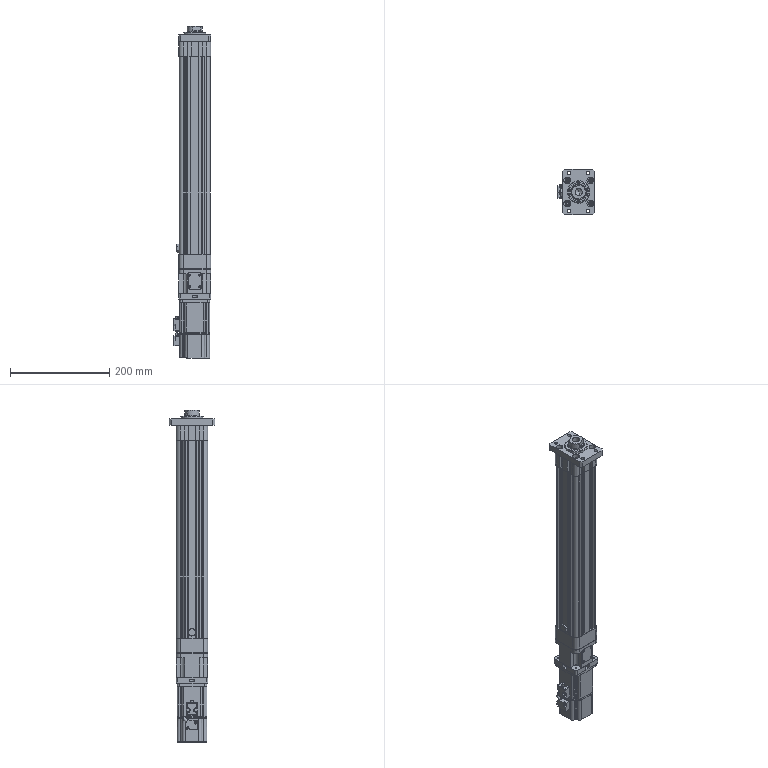Part | SolidWorks | features CompositeCurve 1 | 17 solids | 1083 faces | box 74.85 x 92 x 667.5 mm | volume 1531908 mm3 | cylinder 525 | plane 442 | cone 94 | spline 22 | commonest cylinder face diameters 6 x45 1 x44 8.5 x32 10 x25 0.4 x24 3.3 x24